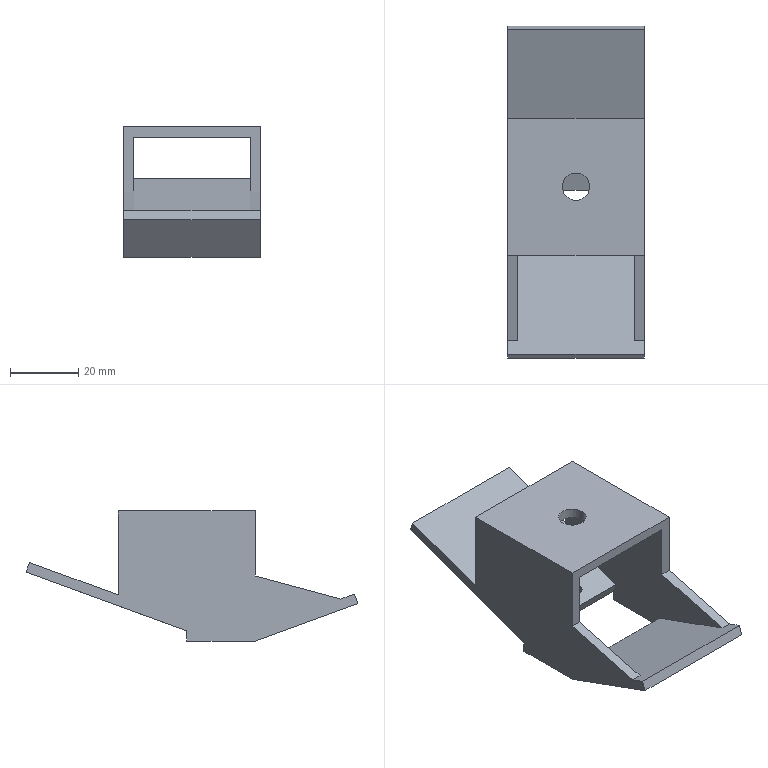Part | STEP file | Blade fixing bracket | 1 solid | 32 faces | box 40 x 96.985 x 38 mm | volume 22805 mm3 | plane 22 | cylinder 10 | commonest cylinder face diameters 2.5 x8 8 x2
STEP:
#1=CARTESIAN_POINT('',(-4.,0.,-1.5));
#2=VERTEX_POINT('',#1);
#3=CARTESIAN_POINT('',(4.,0.,-1.5));
#4=VERTEX_POINT('',#3);
#5=CARTESIAN_POINT('',(0.,0.,-1.5));
#6=DIRECTION('',(0.,0.,1.));
#7=DIRECTION('',(1.,0.,0.));
#8=AXIS2_PLACEMENT_3D('',#5,#6,#7);
#9=CIRCLE('',#8,4.);
#10=EDGE_CURVE('',#2,#4,#9,.T.);
#11=ORIENTED_EDGE('',*,*,#10,.F.);
#12=CARTESIAN_POINT('',(-4.,0.,1.5));
#13=VERTEX_POINT('',#12);
#14=CARTESIAN_POINT('',(-4.,0.,-2.5));
#15=DIRECTION('',(0.,0.,1.));
#16=VECTOR('',#15,1000.);
#17=LINE('',#14,#16);
#18=EDGE_CURVE('',#2,#13,#17,.T.);
#19=ORIENTED_EDGE('',*,*,#18,.T.);
#20=CARTESIAN_POINT('',(4.,0.,1.5));
#21=VERTEX_POINT('',#20);
#22=CARTESIAN_POINT('',(0.,0.,1.5));
#23=DIRECTION('',(0.,0.,1.));
#24=DIRECTION('',(1.,0.,0.));
#25=AXIS2_PLACEMENT_3D('',#22,#23,#24);
#26=CIRCLE('',#25,4.);
#27=EDGE_CURVE('',#13,#21,#26,.T.);
#28=ORIENTED_EDGE('',*,*,#27,.T.);
#29=CARTESIAN_POINT('',(4.,0.,-2.5));
#30=DIRECTION('',(0.,0.,1.));
#31=VECTOR('',#30,1000.);
#32=LINE('',#29,#31);
#33=EDGE_CURVE('',#4,#21,#32,.T.);
#34=ORIENTED_EDGE('',*,*,#33,.F.);
#35=EDGE_LOOP('',(#11,#19,#28,#34));
#36=FACE_OUTER_BOUND('',#35,.T.);
#37=CARTESIAN_POINT('',(0.,0.,-2.5));
#38=DIRECTION('',(0.,0.,1.));
#39=DIRECTION('',(1.,0.,0.));
#40=AXIS2_PLACEMENT_3D('',#37,#38,#39);
#41=CYLINDRICAL_SURFACE('',#40,4.);
#42=ADVANCED_FACE('',(#36),#41,.F.);
#43=CARTESIAN_POINT('',(6.,11.895,-25.978));
#44=VERTEX_POINT('',#43);
#45=CARTESIAN_POINT('',(6.,14.244,-25.123));
#46=VERTEX_POINT('',#45);
#47=CARTESIAN_POINT('',(6.,13.069,-25.551));
#48=DIRECTION('',(0.,0.342,-0.9397));
#49=DIRECTION('',(0.,0.9397,0.342));
#50=AXIS2_PLACEMENT_3D('',#47,#48,#49);
#51=CIRCLE('',#50,1.25);
#52=EDGE_CURVE('',#44,#46,#51,.T.);
#53=ORIENTED_EDGE('',*,*,#52,.F.);
#54=CARTESIAN_POINT('',(6.,12.921,-28.797));
#55=VERTEX_POINT('',#54);
#56=CARTESIAN_POINT('',(6.,12.921,-28.797));
#57=DIRECTION('',(0.,0.342,-0.9397));
#58=VECTOR('',#57,1000.);
#59=LINE('',#56,#58);
#60=EDGE_CURVE('',#44,#55,#59,.T.);
#61=ORIENTED_EDGE('',*,*,#60,.T.);
#62=CARTESIAN_POINT('',(6.,15.27,-27.942));
#63=VERTEX_POINT('',#62);
#64=CARTESIAN_POINT('',(6.,14.095,-28.37));
#65=DIRECTION('',(0.,0.342,-0.9397));
#66=DIRECTION('',(0.,0.9397,0.342));
#67=AXIS2_PLACEMENT_3D('',#64,#65,#66);
#68=CIRCLE('',#67,1.25);
#69=EDGE_CURVE('',#55,#63,#68,.T.);
#70=ORIENTED_EDGE('',*,*,#69,.T.);
#71=CARTESIAN_POINT('',(6.,15.27,-27.942));
#72=DIRECTION('',(0.,0.342,-0.9397));
#73=VECTOR('',#72,1000.);
#74=LINE('',#71,#73);
#75=EDGE_CURVE('',#46,#63,#74,.T.);
#76=ORIENTED_EDGE('',*,*,#75,.F.);
#77=EDGE_LOOP('',(#53,#61,#70,#76));
#78=FACE_OUTER_BOUND('',#77,.T.);
#79=CARTESIAN_POINT('',(6.,14.095,-28.37));
#80=DIRECTION('',(0.,0.342,-0.9397));
#81=DIRECTION('',(0.,0.9397,0.342));
#82=AXIS2_PLACEMENT_3D('',#79,#80,#81);
#83=CYLINDRICAL_SURFACE('',#82,1.25);
#84=ADVANCED_FACE('',(#78),#83,.F.);
#85=CARTESIAN_POINT('',(6.,2.498,-29.398));
#86=VERTEX_POINT('',#85);
#87=CARTESIAN_POINT('',(6.,4.847,-28.543));
#88=VERTEX_POINT('',#87);
#89=CARTESIAN_POINT('',(6.,3.672,-28.971));
#90=DIRECTION('',(0.,0.342,-0.9397));
#91=DIRECTION('',(0.,0.9397,0.342));
#92=AXIS2_PLACEMENT_3D('',#89,#90,#91);
#93=CIRCLE('',#92,1.25);
#94=EDGE_CURVE('',#86,#88,#93,.T.);
#95=ORIENTED_EDGE('',*,*,#94,.F.);
#96=CARTESIAN_POINT('',(6.,3.524,-32.217));
#97=VERTEX_POINT('',#96);
#98=CARTESIAN_POINT('',(6.,3.524,-32.217));
#99=DIRECTION('',(0.,0.342,-0.9397));
#100=VECTOR('',#99,1000.);
#101=LINE('',#98,#100);
#102=EDGE_CURVE('',#86,#97,#101,.T.);
#103=ORIENTED_EDGE('',*,*,#102,.T.);
#104=CARTESIAN_POINT('',(6.,5.873,-31.362));
#105=VERTEX_POINT('',#104);
#106=CARTESIAN_POINT('',(6.,4.698,-31.79));
#107=DIRECTION('',(0.,0.342,-0.9397));
#108=DIRECTION('',(0.,0.9397,0.342));
#109=AXIS2_PLACEMENT_3D('',#106,#107,#108);
#110=CIRCLE('',#109,1.25);
#111=EDGE_CURVE('',#97,#105,#110,.T.);
#112=ORIENTED_EDGE('',*,*,#111,.T.);
#113=CARTESIAN_POINT('',(6.,5.873,-31.362));
#114=DIRECTION('',(0.,0.342,-0.9397));
#115=VECTOR('',#114,1000.);
#116=LINE('',#113,#115);
#117=EDGE_CURVE('',#88,#105,#116,.T.);
#118=ORIENTED_EDGE('',*,*,#117,.F.);
#119=EDGE_LOOP('',(#95,#103,#112,#118));
#120=FACE_OUTER_BOUND('',#119,.T.);
#121=CARTESIAN_POINT('',(6.,4.698,-31.79));
#122=DIRECTION('',(0.,0.342,-0.9397));
#123=DIRECTION('',(0.,0.9397,0.342));
#124=AXIS2_PLACEMENT_3D('',#121,#122,#123);
#125=CYLINDRICAL_SURFACE('',#124,1.25);
#126=ADVANCED_FACE('',(#120),#125,.F.);
#127=CARTESIAN_POINT('',(-6.,2.498,-29.398));
#128=VERTEX_POINT('',#127);
#129=CARTESIAN_POINT('',(-6.,4.847,-28.543));
#130=VERTEX_POINT('',#129);
#131=CARTESIAN_POINT('',(-6.,3.672,-28.971));
#132=DIRECTION('',(0.,0.342,-0.9397));
#133=DIRECTION('',(0.,0.9397,0.342));
#134=AXIS2_PLACEMENT_3D('',#131,#132,#133);
#135=CIRCLE('',#134,1.25);
#136=EDGE_CURVE('',#128,#130,#135,.T.);
#137=ORIENTED_EDGE('',*,*,#136,.F.);
#138=CARTESIAN_POINT('',(-6.,3.524,-32.217));
#139=VERTEX_POINT('',#138);
#140=CARTESIAN_POINT('',(-6.,3.524,-32.217));
#141=DIRECTION('',(0.,0.342,-0.9397));
#142=VECTOR('',#141,1000.);
#143=LINE('',#140,#142);
#144=EDGE_CURVE('',#128,#139,#143,.T.);
#145=ORIENTED_EDGE('',*,*,#144,.T.);
#146=CARTESIAN_POINT('',(-6.,5.873,-31.362));
#147=VERTEX_POINT('',#146);
#148=CARTESIAN_POINT('',(-6.,4.698,-31.79));
#149=DIRECTION('',(0.,0.342,-0.9397));
#150=DIRECTION('',(0.,0.9397,0.342));
#151=AXIS2_PLACEMENT_3D('',#148,#149,#150);
#152=CIRCLE('',#151,1.25);
#153=EDGE_CURVE('',#139,#147,#152,.T.);
#154=ORIENTED_EDGE('',*,*,#153,.T.);
#155=CARTESIAN_POINT('',(-6.,5.873,-31.362));
#156=DIRECTION('',(0.,0.342,-0.9397));
#157=VECTOR('',#156,1000.);
#158=LINE('',#155,#157);
#159=EDGE_CURVE('',#130,#147,#158,.T.);
#160=ORIENTED_EDGE('',*,*,#159,.F.);
#161=EDGE_LOOP('',(#137,#145,#154,#160));
#162=FACE_OUTER_BOUND('',#161,.T.);
#163=CARTESIAN_POINT('',(-6.,4.698,-31.79));
#164=DIRECTION('',(0.,0.342,-0.9397));
#165=DIRECTION('',(0.,0.9397,0.342));
#166=AXIS2_PLACEMENT_3D('',#163,#164,#165);
#167=CYLINDRICAL_SURFACE('',#166,1.25);
#168=ADVANCED_FACE('',(#162),#167,.F.);
#169=CARTESIAN_POINT('',(-6.,11.895,-25.978));
#170=VERTEX_POINT('',#169);
#171=CARTESIAN_POINT('',(-6.,14.244,-25.123));
#172=VERTEX_POINT('',#171);
#173=CARTESIAN_POINT('',(-6.,13.069,-25.551));
#174=DIRECTION('',(0.,0.342,-0.9397));
#175=DIRECTION('',(0.,0.9397,0.342));
#176=AXIS2_PLACEMENT_3D('',#173,#174,#175);
#177=CIRCLE('',#176,1.25);
#178=EDGE_CURVE('',#170,#172,#177,.T.);
#179=ORIENTED_EDGE('',*,*,#178,.F.);
#180=CARTESIAN_POINT('',(-6.,12.921,-28.797));
#181=VERTEX_POINT('',#180);
#182=CARTESIAN_POINT('',(-6.,12.921,-28.797));
#183=DIRECTION('',(0.,0.342,-0.9397));
#184=VECTOR('',#183,1000.);
#185=LINE('',#182,#184);
#186=EDGE_CURVE('',#170,#181,#185,.T.);
#187=ORIENTED_EDGE('',*,*,#186,.T.);
#188=CARTESIAN_POINT('',(-6.,15.27,-27.942));
#189=VERTEX_POINT('',#188);
#190=CARTESIAN_POINT('',(-6.,14.095,-28.37));
#191=DIRECTION('',(0.,0.342,-0.9397));
#192=DIRECTION('',(0.,0.9397,0.342));
#193=AXIS2_PLACEMENT_3D('',#190,#191,#192);
#194=CIRCLE('',#193,1.25);
#195=EDGE_CURVE('',#181,#189,#194,.T.);
#196=ORIENTED_EDGE('',*,*,#195,.T.);
#197=CARTESIAN_POINT('',(-6.,15.27,-27.942));
#198=DIRECTION('',(0.,0.342,-0.9397));
#199=VECTOR('',#198,1000.);
#200=LINE('',#197,#199);
#201=EDGE_CURVE('',#172,#189,#200,.T.);
#202=ORIENTED_EDGE('',*,*,#201,.F.);
#203=EDGE_LOOP('',(#179,#187,#196,#202));
#204=FACE_OUTER_BOUND('',#203,.T.);
#205=CARTESIAN_POINT('',(-6.,14.095,-28.37));
#206=DIRECTION('',(0.,0.342,-0.9397));
#207=DIRECTION('',(0.,0.9397,0.342));
#208=AXIS2_PLACEMENT_3D('',#205,#206,#207);
#209=CYLINDRICAL_SURFACE('',#208,1.25);
#210=ADVANCED_FACE('',(#204),#209,.F.);
#211=CARTESIAN_POINT('',(17.,0.,-33.5));
#212=VERTEX_POINT('',#211);
#213=CARTESIAN_POINT('',(17.,-1.026,-30.681));
#214=VERTEX_POINT('',#213);
#215=CARTESIAN_POINT('',(17.,-1.375,-29.721));
#216=DIRECTION('',(0.,-0.342,0.9397));
#217=VECTOR('',#216,1000.);
#218=LINE('',#215,#217);
#219=EDGE_CURVE('',#212,#214,#218,.T.);
#220=ORIENTED_EDGE('',*,*,#219,.F.);
#221=CARTESIAN_POINT('',(17.,0.,-36.5));
#222=VERTEX_POINT('',#221);
#223=CARTESIAN_POINT('',(17.,0.,-36.5));
#224=DIRECTION('',(0.,0.,-1.));
#225=VECTOR('',#224,1000.);
#226=LINE('',#223,#225);
#227=EDGE_CURVE('',#212,#222,#226,.T.);
#228=ORIENTED_EDGE('',*,*,#227,.T.);
#229=CARTESIAN_POINT('',(17.,-20.,-36.5));
#230=VERTEX_POINT('',#229);
#231=CARTESIAN_POINT('',(17.,-20.,-36.5));
#232=DIRECTION('',(0.,1.,0.));
#233=VECTOR('',#232,1000.);
#234=LINE('',#231,#233);
#235=EDGE_CURVE('',#230,#222,#234,.T.);
#236=ORIENTED_EDGE('',*,*,#235,.F.);
#237=CARTESIAN_POINT('',(17.,-18.974,-33.681));
#238=VERTEX_POINT('',#237);
#239=CARTESIAN_POINT('',(17.,-20.,-36.5));
#240=DIRECTION('',(0.,-0.342,-0.9397));
#241=VECTOR('',#240,1000.);
#242=LINE('',#239,#241);
#243=EDGE_CURVE('',#238,#230,#242,.T.);
#244=ORIENTED_EDGE('',*,*,#243,.F.);
#245=CARTESIAN_POINT('',(17.,-44.959,-24.223));
#246=VERTEX_POINT('',#245);
#247=CARTESIAN_POINT('',(17.,-18.974,-33.681));
#248=DIRECTION('',(0.,0.9397,-0.342));
#249=VECTOR('',#248,1000.);
#250=LINE('',#247,#249);
#251=EDGE_CURVE('',#246,#238,#250,.T.);
#252=ORIENTED_EDGE('',*,*,#251,.F.);
#253=CARTESIAN_POINT('',(17.,-20.,-17.5));
#254=VERTEX_POINT('',#253);
#255=CARTESIAN_POINT('',(17.,-50.,-25.581));
#256=DIRECTION('',(0.,-0.9656,-0.2601));
#257=VECTOR('',#256,1000.);
#258=LINE('',#255,#257);
#259=EDGE_CURVE('',#254,#246,#258,.T.);
#260=ORIENTED_EDGE('',*,*,#259,.F.);
#261=CARTESIAN_POINT('',(17.,-20.,-1.5));
#262=VERTEX_POINT('',#261);
#263=CARTESIAN_POINT('',(17.,-20.,-36.5));
#264=DIRECTION('',(0.,0.,1.));
#265=VECTOR('',#264,1000.);
#266=LINE('',#263,#265);
#267=EDGE_CURVE('',#254,#262,#266,.T.);
#268=ORIENTED_EDGE('',*,*,#267,.T.);
#269=CARTESIAN_POINT('',(17.,20.,-1.5));
#270=VERTEX_POINT('',#269);
#271=CARTESIAN_POINT('',(17.,-20.,-1.5));
#272=DIRECTION('',(0.,1.,0.));
#273=VECTOR('',#272,1000.);
#274=LINE('',#271,#273);
#275=EDGE_CURVE('',#262,#270,#274,.T.);
#276=ORIENTED_EDGE('',*,*,#275,.T.);
#277=CARTESIAN_POINT('',(17.,20.,-23.028));
#278=VERTEX_POINT('',#277);
#279=CARTESIAN_POINT('',(17.,20.,-36.5));
#280=DIRECTION('',(0.,0.,1.));
#281=VECTOR('',#280,1000.);
#282=LINE('',#279,#281);
#283=EDGE_CURVE('',#278,#270,#282,.T.);
#284=ORIENTED_EDGE('',*,*,#283,.F.);
#285=CARTESIAN_POINT('',(17.,-19.651,-37.46));
#286=DIRECTION('',(0.,0.9397,0.342));
#287=VECTOR('',#286,1000.);
#288=LINE('',#285,#287);
#289=EDGE_CURVE('',#214,#278,#288,.T.);
#290=ORIENTED_EDGE('',*,*,#289,.F.);
#291=EDGE_LOOP('',(#220,#228,#236,#244,#252,#260,#268,#276,#284,#290));
#292=FACE_OUTER_BOUND('',#291,.T.);
#293=CARTESIAN_POINT('',(17.,-20.,-36.5));
#294=DIRECTION('',(1.,0.,0.));
#295=DIRECTION('',(0.,0.,-1.));
#296=AXIS2_PLACEMENT_3D('',#293,#294,#295);
#297=PLANE('',#296);
#298=ADVANCED_FACE('',(#292),#297,.F.);
#299=CARTESIAN_POINT('',(-17.,0.,-36.5));
#300=VERTEX_POINT('',#299);
#301=CARTESIAN_POINT('',(-17.,-20.,-36.5));
#302=VERTEX_POINT('',#301);
#303=CARTESIAN_POINT('',(-17.,-20.,-36.5));
#304=DIRECTION('',(0.,-1.,0.));
#305=VECTOR('',#304,1000.);
#306=LINE('',#303,#305);
#307=EDGE_CURVE('',#300,#302,#306,.T.);
#308=ORIENTED_EDGE('',*,*,#307,.F.);
#309=CARTESIAN_POINT('',(-17.,0.,-33.5));
#310=VERTEX_POINT('',#309);
#311=CARTESIAN_POINT('',(-17.,0.,-36.5));
#312=DIRECTION('',(0.,0.,1.));
#313=VECTOR('',#312,1000.);
#314=LINE('',#311,#313);
#315=EDGE_CURVE('',#300,#310,#314,.T.);
#316=ORIENTED_EDGE('',*,*,#315,.T.);
#317=CARTESIAN_POINT('',(-17.,-1.026,-30.681));
#318=VERTEX_POINT('',#317);
#319=CARTESIAN_POINT('',(-17.,-1.375,-29.721));
#320=DIRECTION('',(0.,0.342,-0.9397));
#321=VECTOR('',#320,1000.);
#322=LINE('',#319,#321);
#323=EDGE_CURVE('',#318,#310,#322,.T.);
#324=ORIENTED_EDGE('',*,*,#323,.F.);
#325=CARTESIAN_POINT('',(-17.,20.,-23.028));
#326=VERTEX_POINT('',#325);
#327=CARTESIAN_POINT('',(-17.,-19.651,-37.46));
#328=DIRECTION('',(0.,-0.9397,-0.342));
#329=VECTOR('',#328,1000.);
#330=LINE('',#327,#329);
#331=EDGE_CURVE('',#326,#318,#330,.T.);
#332=ORIENTED_EDGE('',*,*,#331,.F.);
#333=CARTESIAN_POINT('',(-17.,20.,-1.5));
#334=VERTEX_POINT('',#333);
#335=CARTESIAN_POINT('',(-17.,20.,-36.5));
#336=DIRECTION('',(0.,0.,1.));
#337=VECTOR('',#336,1000.);
#338=LINE('',#335,#337);
#339=EDGE_CURVE('',#326,#334,#338,.T.);
#340=ORIENTED_EDGE('',*,*,#339,.T.);
#341=CARTESIAN_POINT('',(-17.,-20.,-1.5));
#342=VERTEX_POINT('',#341);
#343=CARTESIAN_POINT('',(-17.,-20.,-1.5));
#344=DIRECTION('',(0.,-1.,0.));
#345=VECTOR('',#344,1000.);
#346=LINE('',#343,#345);
#347=EDGE_CURVE('',#334,#342,#346,.T.);
#348=ORIENTED_EDGE('',*,*,#347,.T.);
#349=CARTESIAN_POINT('',(-17.,-20.,-17.5));
#350=VERTEX_POINT('',#349);
#351=CARTESIAN_POINT('',(-17.,-20.,-36.5));
#352=DIRECTION('',(0.,0.,1.));
#353=VECTOR('',#352,1000.);
#354=LINE('',#351,#353);
#355=EDGE_CURVE('',#350,#342,#354,.T.);
#356=ORIENTED_EDGE('',*,*,#355,.F.);
#357=CARTESIAN_POINT('',(-17.,-44.959,-24.223));
#358=VERTEX_POINT('',#357);
#359=CARTESIAN_POINT('',(-17.,-50.,-25.581));
#360=DIRECTION('',(0.,-0.9656,-0.2601));
#361=VECTOR('',#360,1000.);
#362=LINE('',#359,#361);
#363=EDGE_CURVE('',#350,#358,#362,.T.);
#364=ORIENTED_EDGE('',*,*,#363,.T.);
#365=CARTESIAN_POINT('',(-17.,-18.974,-33.681));
#366=VERTEX_POINT('',#365);
#367=CARTESIAN_POINT('',(-17.,-18.974,-33.681));
#368=DIRECTION('',(0.,-0.9397,0.342));
#369=VECTOR('',#368,1000.);
#370=LINE('',#367,#369);
#371=EDGE_CURVE('',#366,#358,#370,.T.);
#372=ORIENTED_EDGE('',*,*,#371,.F.);
#373=CARTESIAN_POINT('',(-17.,-20.,-36.5));
#374=DIRECTION('',(0.,0.342,0.9397));
#375=VECTOR('',#374,1000.);
#376=LINE('',#373,#375);
#377=EDGE_CURVE('',#302,#366,#376,.T.);
#378=ORIENTED_EDGE('',*,*,#377,.F.);
#379=EDGE_LOOP('',(#308,#316,#324,#332,#340,#348,#356,#364,#372,#378));
#380=FACE_OUTER_BOUND('',#379,.T.);
#381=CARTESIAN_POINT('',(-17.,-20.,-36.5));
#382=DIRECTION('',(-1.,0.,0.));
#383=DIRECTION('',(0.,0.,1.));
#384=AXIS2_PLACEMENT_3D('',#381,#382,#383);
#385=PLANE('',#384);
#386=ADVANCED_FACE('',(#380),#385,.F.);
#387=CARTESIAN_POINT('',(-20.,20.,-23.028));
#388=VERTEX_POINT('',#387);
#389=CARTESIAN_POINT('',(-20.,20.,-23.028));
#390=DIRECTION('',(1.,0.,0.));
#391=VECTOR('',#390,1000.);
#392=LINE('',#389,#391);
#393=EDGE_CURVE('',#388,#326,#392,.T.);
#394=ORIENTED_EDGE('',*,*,#393,.F.);
#395=CARTESIAN_POINT('',(-20.,20.,1.5));
#396=VERTEX_POINT('',#395);
#397=CARTESIAN_POINT('',(-20.,20.,1.5));
#398=DIRECTION('',(0.,0.,-1.));
#399=VECTOR('',#398,1000.);
#400=LINE('',#397,#399);
#401=EDGE_CURVE('',#396,#388,#400,.T.);
#402=ORIENTED_EDGE('',*,*,#401,.F.);
#403=CARTESIAN_POINT('',(20.,20.,1.5));
#404=VERTEX_POINT('',#403);
#405=CARTESIAN_POINT('',(-20.,20.,1.5));
#406=DIRECTION('',(-1.,0.,0.));
#407=VECTOR('',#406,1000.);
#408=LINE('',#405,#407);
#409=EDGE_CURVE('',#404,#396,#408,.T.);
#410=ORIENTED_EDGE('',*,*,#409,.F.);
#411=CARTESIAN_POINT('',(20.,20.,-23.028));
#412=VERTEX_POINT('',#411);
#413=CARTESIAN_POINT('',(20.,20.,1.5));
#414=DIRECTION('',(0.,0.,-1.));
#415=VECTOR('',#414,1000.);
#416=LINE('',#413,#415);
#417=EDGE_CURVE('',#404,#412,#416,.T.);
#418=ORIENTED_EDGE('',*,*,#417,.T.);
#419=CARTESIAN_POINT('',(-20.,20.,-23.028));
#420=DIRECTION('',(1.,0.,0.));
#421=VECTOR('',#420,1000.);
#422=LINE('',#419,#421);
#423=EDGE_CURVE('',#278,#412,#422,.T.);
#424=ORIENTED_EDGE('',*,*,#423,.F.);
#425=ORIENTED_EDGE('',*,*,#283,.T.);
#426=CARTESIAN_POINT('',(-20.,20.,-1.5));
#427=DIRECTION('',(-1.,0.,0.));
#428=VECTOR('',#427,1000.);
#429=LINE('',#426,#428);
#430=EDGE_CURVE('',#270,#334,#429,.T.);
#431=ORIENTED_EDGE('',*,*,#430,.T.);
#432=ORIENTED_EDGE('',*,*,#339,.F.);
#433=EDGE_LOOP('',(#394,#402,#410,#418,#424,#425,#431,#432));
#434=FACE_OUTER_BOUND('',#433,.T.);
#435=CARTESIAN_POINT('',(-20.,20.,1.5));
#436=DIRECTION('',(0.,-1.,0.));
#437=DIRECTION('',(0.,0.,-1.));
#438=AXIS2_PLACEMENT_3D('',#435,#436,#437);
#439=PLANE('',#438);
#440=ADVANCED_FACE('',(#434),#439,.F.);
#441=ORIENTED_EDGE('',*,*,#259,.T.);
#442=CARTESIAN_POINT('',(20.,-44.959,-24.223));
#443=VERTEX_POINT('',#442);
#444=CARTESIAN_POINT('',(17.,-44.959,-24.223));
#445=DIRECTION('',(1.,0.,0.));
#446=VECTOR('',#445,1000.);
#447=LINE('',#444,#446);
#448=EDGE_CURVE('',#246,#443,#447,.T.);
#449=ORIENTED_EDGE('',*,*,#448,.T.);
#450=CARTESIAN_POINT('',(20.,-20.,-17.5));
#451=VERTEX_POINT('',#450);
#452=CARTESIAN_POINT('',(20.,-50.,-25.581));
#453=DIRECTION('',(0.,-0.9656,-0.2601));
#454=VECTOR('',#453,1000.);
#455=LINE('',#452,#454);
#456=EDGE_CURVE('',#451,#443,#455,.T.);
#457=ORIENTED_EDGE('',*,*,#456,.F.);
#458=CARTESIAN_POINT('',(17.,-20.,-17.5));
#459=DIRECTION('',(1.,0.,0.));
#460=VECTOR('',#459,1000.);
#461=LINE('',#458,#460);
#462=EDGE_CURVE('',#254,#451,#461,.T.);
#463=ORIENTED_EDGE('',*,*,#462,.F.);
#464=EDGE_LOOP('',(#441,#449,#457,#463));
#465=FACE_OUTER_BOUND('',#464,.T.);
#466=CARTESIAN_POINT('',(17.,-50.,-25.581));
#467=DIRECTION('',(0.,-0.2601,0.9656));
#468=DIRECTION('',(0.,-0.9656,-0.2601));
#469=AXIS2_PLACEMENT_3D('',#466,#467,#468);
#470=PLANE('',#469);
#471=ADVANCED_FACE('',(#465),#470,.T.);
#472=CARTESIAN_POINT('',(-20.,-44.959,-24.223));
#473=VERTEX_POINT('',#472);
#474=CARTESIAN_POINT('',(-17.,-44.959,-24.223));
#475=DIRECTION('',(-1.,0.,0.));
#476=VECTOR('',#475,1000.);
#477=LINE('',#474,#476);
#478=EDGE_CURVE('',#358,#473,#477,.T.);
#479=ORIENTED_EDGE('',*,*,#478,.F.);
#480=ORIENTED_EDGE('',*,*,#363,.F.);
#481=CARTESIAN_POINT('',(-20.,-20.,-17.5));
#482=VERTEX_POINT('',#481);
#483=CARTESIAN_POINT('',(-17.,-20.,-17.5));
#484=DIRECTION('',(-1.,0.,0.));
#485=VECTOR('',#484,1000.);
#486=LINE('',#483,#485);
#487=EDGE_CURVE('',#350,#482,#486,.T.);
#488=ORIENTED_EDGE('',*,*,#487,.T.);
#489=CARTESIAN_POINT('',(-20.,-50.,-25.581));
#490=DIRECTION('',(0.,-0.9656,-0.2601));
#491=VECTOR('',#490,1000.);
#492=LINE('',#489,#491);
#493=EDGE_CURVE('',#482,#473,#492,.T.);
#494=ORIENTED_EDGE('',*,*,#493,.T.);
#495=EDGE_LOOP('',(#479,#480,#488,#494));
#496=FACE_OUTER_BOUND('',#495,.T.);
#497=CARTESIAN_POINT('',(-17.,-50.,-25.581));
#498=DIRECTION('',(0.,0.2601,-0.9656));
#499=DIRECTION('',(0.,0.9656,0.2601));
#500=AXIS2_PLACEMENT_3D('',#497,#498,#499);
#501=PLANE('',#500);
#502=ADVANCED_FACE('',(#496),#501,.F.);
#503=ORIENTED_EDGE('',*,*,#487,.F.);
#504=ORIENTED_EDGE('',*,*,#355,.T.);
#505=CARTESIAN_POINT('',(-20.,-20.,-1.5));
#506=DIRECTION('',(1.,0.,0.));
#507=VECTOR('',#506,1000.);
#508=LINE('',#505,#507);
#509=EDGE_CURVE('',#342,#262,#508,.T.);
#510=ORIENTED_EDGE('',*,*,#509,.T.);
#511=ORIENTED_EDGE('',*,*,#267,.F.);
#512=ORIENTED_EDGE('',*,*,#462,.T.);
#513=CARTESIAN_POINT('',(20.,-20.,1.5));
#514=VERTEX_POINT('',#513);
#515=CARTESIAN_POINT('',(20.,-20.,1.5));
#516=DIRECTION('',(0.,0.,-1.));
#517=VECTOR('',#516,1000.);
#518=LINE('',#515,#517);
#519=EDGE_CURVE('',#514,#451,#518,.T.);
#520=ORIENTED_EDGE('',*,*,#519,.F.);
#521=CARTESIAN_POINT('',(-20.,-20.,1.5));
#522=VERTEX_POINT('',#521);
#523=CARTESIAN_POINT('',(-20.,-20.,1.5));
#524=DIRECTION('',(1.,0.,0.));
#525=VECTOR('',#524,1000.);
#526=LINE('',#523,#525);
#527=EDGE_CURVE('',#522,#514,#526,.T.);
#528=ORIENTED_EDGE('',*,*,#527,.F.);
#529=CARTESIAN_POINT('',(-20.,-20.,1.5));
#530=DIRECTION('',(0.,0.,-1.));
#531=VECTOR('',#530,1000.);
#532=LINE('',#529,#531);
#533=EDGE_CURVE('',#522,#482,#532,.T.);
#534=ORIENTED_EDGE('',*,*,#533,.T.);
#535=EDGE_LOOP('',(#503,#504,#510,#511,#512,#520,#528,#534));
#536=FACE_OUTER_BOUND('',#535,.T.);
#537=CARTESIAN_POINT('',(-20.,-20.,1.5));
#538=DIRECTION('',(0.,1.,0.));
#539=DIRECTION('',(0.,0.,1.));
#540=AXIS2_PLACEMENT_3D('',#537,#538,#539);
#541=PLANE('',#540);
#542=ADVANCED_FACE('',(#536),#541,.F.);
#543=CARTESIAN_POINT('',(0.,0.,-1.5));
#544=DIRECTION('',(0.,0.,1.));
#545=DIRECTION('',(1.,0.,0.));
#546=AXIS2_PLACEMENT_3D('',#543,#544,#545);
#547=CIRCLE('',#546,4.);
#548=EDGE_CURVE('',#4,#2,#547,.T.);
#549=ORIENTED_EDGE('',*,*,#548,.T.);
#550=ORIENTED_EDGE('',*,*,#10,.T.);
#551=EDGE_LOOP('',(#549,#550));
#552=FACE_BOUND('',#551,.T.);
#553=ORIENTED_EDGE('',*,*,#347,.F.);
#554=ORIENTED_EDGE('',*,*,#430,.F.);
#555=ORIENTED_EDGE('',*,*,#275,.F.);
#556=ORIENTED_EDGE('',*,*,#509,.F.);
#557=EDGE_LOOP('',(#553,#554,#555,#556));
#558=FACE_OUTER_BOUND('',#557,.T.);
#559=CARTESIAN_POINT('',(0.,0.,-1.5));
#560=DIRECTION('',(0.,0.,1.));
#561=DIRECTION('',(1.,0.,0.));
#562=AXIS2_PLACEMENT_3D('',#559,#560,#561);
#563=PLANE('',#562);
#564=ADVANCED_FACE('',(#552,#558),#563,.F.);
#565=CARTESIAN_POINT('',(20.,0.,-36.5));
#566=VERTEX_POINT('',#565);
#567=CARTESIAN_POINT('',(20.,0.,-33.5));
#568=VERTEX_POINT('',#567);
#569=CARTESIAN_POINT('',(20.,0.,1.5));
#570=DIRECTION('',(0.,0.,1.));
#571=VECTOR('',#570,1000.);
#572=LINE('',#569,#571);
#573=EDGE_CURVE('',#566,#568,#572,.T.);
#574=ORIENTED_EDGE('',*,*,#573,.T.);
#575=CARTESIAN_POINT('',(20.,46.985,-16.399));
#576=VERTEX_POINT('',#575);
#577=CARTESIAN_POINT('',(20.,46.985,-16.399));
#578=DIRECTION('',(0.,-0.9397,-0.342));
#579=VECTOR('',#578,1000.);
#580=LINE('',#577,#579);
#581=EDGE_CURVE('',#576,#568,#580,.T.);
#582=ORIENTED_EDGE('',*,*,#581,.F.);
#583=CARTESIAN_POINT('',(20.,45.959,-13.58));
#584=VERTEX_POINT('',#583);
#585=CARTESIAN_POINT('',(20.,45.959,-13.58));
#586=DIRECTION('',(0.,0.342,-0.9397));
#587=VECTOR('',#586,1000.);
#588=LINE('',#585,#587);
#589=EDGE_CURVE('',#584,#576,#588,.T.);
#590=ORIENTED_EDGE('',*,*,#589,.F.);
#591=CARTESIAN_POINT('',(20.,-1.026,-30.681));
#592=DIRECTION('',(0.,0.9397,0.342));
#593=VECTOR('',#592,1000.);
#594=LINE('',#591,#593);
#595=EDGE_CURVE('',#412,#584,#594,.T.);
#596=ORIENTED_EDGE('',*,*,#595,.F.);
#597=ORIENTED_EDGE('',*,*,#417,.F.);
#598=CARTESIAN_POINT('',(20.,20.,1.5));
#599=DIRECTION('',(0.,1.,0.));
#600=VECTOR('',#599,1000.);
#601=LINE('',#598,#600);
#602=EDGE_CURVE('',#514,#404,#601,.T.);
#603=ORIENTED_EDGE('',*,*,#602,.F.);
#604=ORIENTED_EDGE('',*,*,#519,.T.);
#605=ORIENTED_EDGE('',*,*,#456,.T.);
#606=CARTESIAN_POINT('',(20.,-48.974,-22.762));
#607=VERTEX_POINT('',#606);
#608=CARTESIAN_POINT('',(20.,-48.974,-22.762));
#609=DIRECTION('',(0.,-0.9397,0.342));
#610=VECTOR('',#609,1000.);
#611=LINE('',#608,#610);
#612=EDGE_CURVE('',#443,#607,#611,.T.);
#613=ORIENTED_EDGE('',*,*,#612,.T.);
#614=CARTESIAN_POINT('',(20.,-50.,-25.581));
#615=VERTEX_POINT('',#614);
#616=CARTESIAN_POINT('',(20.,-48.974,-22.762));
#617=DIRECTION('',(0.,-0.342,-0.9397));
#618=VECTOR('',#617,1000.);
#619=LINE('',#616,#618);
#620=EDGE_CURVE('',#607,#615,#619,.T.);
#621=ORIENTED_EDGE('',*,*,#620,.T.);
#622=CARTESIAN_POINT('',(20.,-20.,-36.5));
#623=VERTEX_POINT('',#622);
#624=CARTESIAN_POINT('',(20.,-20.,-36.5));
#625=DIRECTION('',(0.,0.9397,-0.342));
#626=VECTOR('',#625,1000.);
#627=LINE('',#624,#626);
#628=EDGE_CURVE('',#615,#623,#627,.T.);
#629=ORIENTED_EDGE('',*,*,#628,.T.);
#630=CARTESIAN_POINT('',(20.,-20.,-36.5));
#631=DIRECTION('',(0.,-1.,0.));
#632=VECTOR('',#631,1000.);
#633=LINE('',#630,#632);
#634=EDGE_CURVE('',#566,#623,#633,.T.);
#635=ORIENTED_EDGE('',*,*,#634,.F.);
#636=EDGE_LOOP('',(#574,#582,#590,#596,#597,#603,#604,#605,#613,#621,#629,#635));
#637=FACE_OUTER_BOUND('',#636,.T.);
#638=CARTESIAN_POINT('',(20.,20.,1.5));
#639=DIRECTION('',(-1.,0.,0.));
#640=DIRECTION('',(0.,-1.,0.));
#641=AXIS2_PLACEMENT_3D('',#638,#639,#640);
#642=PLANE('',#641);
#643=ADVANCED_FACE('',(#637),#642,.F.);
#644=CARTESIAN_POINT('',(-20.,0.,-33.5));
#645=VERTEX_POINT('',#644);
#646=CARTESIAN_POINT('',(-20.,46.985,-16.399));
#647=VERTEX_POINT('',#646);
#648=CARTESIAN_POINT('',(-20.,0.,-33.5));
#649=DIRECTION('',(0.,0.9397,0.342));
#650=VECTOR('',#649,1000.);
#651=LINE('',#648,#650);
#652=EDGE_CURVE('',#645,#647,#651,.T.);
#653=ORIENTED_EDGE('',*,*,#652,.F.);
#654=CARTESIAN_POINT('',(-20.,0.,-36.5));
#655=VERTEX_POINT('',#654);
#656=CARTESIAN_POINT('',(-20.,0.,1.5));
#657=DIRECTION('',(0.,0.,-1.));
#658=VECTOR('',#657,1000.);
#659=LINE('',#656,#658);
#660=EDGE_CURVE('',#645,#655,#659,.T.);
#661=ORIENTED_EDGE('',*,*,#660,.T.);
#662=CARTESIAN_POINT('',(-20.,-20.,-36.5));
#663=VERTEX_POINT('',#662);
#664=CARTESIAN_POINT('',(-20.,-20.,-36.5));
#665=DIRECTION('',(0.,1.,0.));
#666=VECTOR('',#665,1000.);
#667=LINE('',#664,#666);
#668=EDGE_CURVE('',#663,#655,#667,.T.);
#669=ORIENTED_EDGE('',*,*,#668,.F.);
#670=CARTESIAN_POINT('',(-20.,-50.,-25.581));
#671=VERTEX_POINT('',#670);
#672=CARTESIAN_POINT('',(-20.,-20.,-36.5));
#673=DIRECTION('',(0.,0.9397,-0.342));
#674=VECTOR('',#673,1000.);
#675=LINE('',#672,#674);
#676=EDGE_CURVE('',#671,#663,#675,.T.);
#677=ORIENTED_EDGE('',*,*,#676,.F.);
#678=CARTESIAN_POINT('',(-20.,-48.974,-22.762));
#679=VERTEX_POINT('',#678);
#680=CARTESIAN_POINT('',(-20.,-48.974,-22.762));
#681=DIRECTION('',(0.,-0.342,-0.9397));
#682=VECTOR('',#681,1000.);
#683=LINE('',#680,#682);
#684=EDGE_CURVE('',#679,#671,#683,.T.);
#685=ORIENTED_EDGE('',*,*,#684,.F.);
#686=CARTESIAN_POINT('',(-20.,-48.974,-22.762));
#687=DIRECTION('',(0.,-0.9397,0.342));
#688=VECTOR('',#687,1000.);
#689=LINE('',#686,#688);
#690=EDGE_CURVE('',#473,#679,#689,.T.);
#691=ORIENTED_EDGE('',*,*,#690,.F.);
#692=ORIENTED_EDGE('',*,*,#493,.F.);
#693=ORIENTED_EDGE('',*,*,#533,.F.);
#694=CARTESIAN_POINT('',(-20.,20.,1.5));
#695=DIRECTION('',(0.,-1.,0.));
#696=VECTOR('',#695,1000.);
#697=LINE('',#694,#696);
#698=EDGE_CURVE('',#396,#522,#697,.T.);
#699=ORIENTED_EDGE('',*,*,#698,.F.);
#700=ORIENTED_EDGE('',*,*,#401,.T.);
#701=CARTESIAN_POINT('',(-20.,45.959,-13.58));
#702=VERTEX_POINT('',#701);
#703=CARTESIAN_POINT('',(-20.,-1.026,-30.681));
#704=DIRECTION('',(0.,-0.9397,-0.342));
#705=VECTOR('',#704,1000.);
#706=LINE('',#703,#705);
#707=EDGE_CURVE('',#702,#388,#706,.T.);
#708=ORIENTED_EDGE('',*,*,#707,.F.);
#709=CARTESIAN_POINT('',(-20.,45.959,-13.58));
#710=DIRECTION('',(0.,-0.342,0.9397));
#711=VECTOR('',#710,1000.);
#712=LINE('',#709,#711);
#713=EDGE_CURVE('',#647,#702,#712,.T.);
#714=ORIENTED_EDGE('',*,*,#713,.F.);
#715=EDGE_LOOP('',(#653,#661,#669,#677,#685,#691,#692,#693,#699,#700,#708,#714));
#716=FACE_OUTER_BOUND('',#715,.T.);
#717=CARTESIAN_POINT('',(-20.,20.,1.5));
#718=DIRECTION('',(1.,0.,0.));
#719=DIRECTION('',(0.,1.,0.));
#720=AXIS2_PLACEMENT_3D('',#717,#718,#719);
#721=PLANE('',#720);
#722=ADVANCED_FACE('',(#716),#721,.F.);
#723=CARTESIAN_POINT('',(0.,0.,1.5));
#724=DIRECTION('',(0.,0.,1.));
#725=DIRECTION('',(1.,0.,0.));
#726=AXIS2_PLACEMENT_3D('',#723,#724,#725);
#727=CIRCLE('',#726,4.);
#728=EDGE_CURVE('',#21,#13,#727,.T.);
#729=ORIENTED_EDGE('',*,*,#728,.F.);
#730=ORIENTED_EDGE('',*,*,#27,.F.);
#731=EDGE_LOOP('',(#729,#730));
#732=FACE_BOUND('',#731,.T.);
#733=ORIENTED_EDGE('',*,*,#602,.T.);
#734=ORIENTED_EDGE('',*,*,#409,.T.);
#735=ORIENTED_EDGE('',*,*,#698,.T.);
#736=ORIENTED_EDGE('',*,*,#527,.T.);
#737=EDGE_LOOP('',(#733,#734,#735,#736));
#738=FACE_OUTER_BOUND('',#737,.T.);
#739=CARTESIAN_POINT('',(0.,0.,1.5));
#740=DIRECTION('',(0.,0.,1.));
#741=DIRECTION('',(1.,0.,0.));
#742=AXIS2_PLACEMENT_3D('',#739,#740,#741);
#743=PLANE('',#742);
#744=ADVANCED_FACE('',(#732,#738),#743,.T.);
#745=ORIENTED_EDGE('',*,*,#235,.T.);
#746=CARTESIAN_POINT('',(0.,0.,-36.5));
#747=DIRECTION('',(1.,0.,0.));
#748=VECTOR('',#747,1000.);
#749=LINE('',#746,#748);
#750=EDGE_CURVE('',#222,#566,#749,.T.);
#751=ORIENTED_EDGE('',*,*,#750,.T.);
#752=ORIENTED_EDGE('',*,*,#634,.T.);
#753=CARTESIAN_POINT('',(20.,-20.,-36.5));
#754=DIRECTION('',(-1.,0.,0.));
#755=VECTOR('',#754,1000.);
#756=LINE('',#753,#755);
#757=EDGE_CURVE('',#623,#230,#756,.T.);
#758=ORIENTED_EDGE('',*,*,#757,.T.);
#759=EDGE_LOOP('',(#745,#751,#752,#758));
#760=FACE_OUTER_BOUND('',#759,.T.);
#761=CARTESIAN_POINT('',(0.,0.,-36.5));
#762=DIRECTION('',(0.,0.,1.));
#763=DIRECTION('',(1.,0.,0.));
#764=AXIS2_PLACEMENT_3D('',#761,#762,#763);
#765=PLANE('',#764);
#766=ADVANCED_FACE('',(#760),#765,.F.);
#767=CARTESIAN_POINT('',(0.,0.,-36.5));
#768=DIRECTION('',(-1.,0.,0.));
#769=VECTOR('',#768,1000.);
#770=LINE('',#767,#769);
#771=EDGE_CURVE('',#300,#655,#770,.T.);
#772=ORIENTED_EDGE('',*,*,#771,.F.);
#773=ORIENTED_EDGE('',*,*,#307,.T.);
#774=CARTESIAN_POINT('',(-20.,-20.,-36.5));
#775=DIRECTION('',(-1.,0.,0.));
#776=VECTOR('',#775,1000.);
#777=LINE('',#774,#776);
#778=EDGE_CURVE('',#302,#663,#777,.T.);
#779=ORIENTED_EDGE('',*,*,#778,.T.);
#780=ORIENTED_EDGE('',*,*,#668,.T.);
#781=EDGE_LOOP('',(#772,#773,#779,#780));
#782=FACE_OUTER_BOUND('',#781,.T.);
#783=CARTESIAN_POINT('',(0.,0.,-36.5));
#784=DIRECTION('',(0.,0.,-1.));
#785=DIRECTION('',(-1.,0.,0.));
#786=AXIS2_PLACEMENT_3D('',#783,#784,#785);
#787=PLANE('',#786);
#788=ADVANCED_FACE('',(#782),#787,.T.);
#789=ORIENTED_EDGE('',*,*,#628,.F.);
#790=CARTESIAN_POINT('',(17.,-50.,-25.581));
#791=DIRECTION('',(1.,0.,0.));
#792=VECTOR('',#791,1000.);
#793=LINE('',#790,#792);
#794=EDGE_CURVE('',#671,#615,#793,.T.);
#795=ORIENTED_EDGE('',*,*,#794,.F.);
#796=ORIENTED_EDGE('',*,*,#676,.T.);
#797=ORIENTED_EDGE('',*,*,#778,.F.);
#798=CARTESIAN_POINT('',(20.,-20.,-36.5));
#799=DIRECTION('',(-1.,0.,0.));
#800=VECTOR('',#799,1000.);
#801=LINE('',#798,#800);
#802=EDGE_CURVE('',#230,#302,#801,.T.);
#803=ORIENTED_EDGE('',*,*,#802,.F.);
#804=ORIENTED_EDGE('',*,*,#757,.F.);
#805=EDGE_LOOP('',(#789,#795,#796,#797,#803,#804));
#806=FACE_OUTER_BOUND('',#805,.T.);
#807=CARTESIAN_POINT('',(17.,-20.,-36.5));
#808=DIRECTION('',(0.,-0.342,-0.9397));
#809=DIRECTION('',(0.,0.9397,-0.342));
#810=AXIS2_PLACEMENT_3D('',#807,#808,#809);
#811=PLANE('',#810);
#812=ADVANCED_FACE('',(#806),#811,.T.);
#813=ORIENTED_EDGE('',*,*,#448,.F.);
#814=ORIENTED_EDGE('',*,*,#251,.T.);
#815=CARTESIAN_POINT('',(20.,-18.974,-33.681));
#816=DIRECTION('',(-1.,0.,0.));
#817=VECTOR('',#816,1000.);
#818=LINE('',#815,#817);
#819=EDGE_CURVE('',#238,#366,#818,.T.);
#820=ORIENTED_EDGE('',*,*,#819,.T.);
#821=ORIENTED_EDGE('',*,*,#371,.T.);
#822=ORIENTED_EDGE('',*,*,#478,.T.);
#823=ORIENTED_EDGE('',*,*,#690,.T.);
#824=CARTESIAN_POINT('',(20.,-48.974,-22.762));
#825=DIRECTION('',(-1.,0.,0.));
#826=VECTOR('',#825,1000.);
#827=LINE('',#824,#826);
#828=EDGE_CURVE('',#607,#679,#827,.T.);
#829=ORIENTED_EDGE('',*,*,#828,.F.);
#830=ORIENTED_EDGE('',*,*,#612,.F.);
#831=EDGE_LOOP('',(#813,#814,#820,#821,#822,#823,#829,#830));
#832=FACE_OUTER_BOUND('',#831,.T.);
#833=CARTESIAN_POINT('',(20.,-48.974,-22.762));
#834=DIRECTION('',(0.,-0.342,-0.9397));
#835=DIRECTION('',(0.,0.9397,-0.342));
#836=AXIS2_PLACEMENT_3D('',#833,#834,#835);
#837=PLANE('',#836);
#838=ADVANCED_FACE('',(#832),#837,.F.);
#839=ORIENTED_EDGE('',*,*,#819,.F.);
#840=ORIENTED_EDGE('',*,*,#243,.T.);
#841=ORIENTED_EDGE('',*,*,#802,.T.);
#842=ORIENTED_EDGE('',*,*,#377,.T.);
#843=EDGE_LOOP('',(#839,#840,#841,#842));
#844=FACE_OUTER_BOUND('',#843,.T.);
#845=CARTESIAN_POINT('',(20.,-18.974,-33.681));
#846=DIRECTION('',(0.,-0.9397,0.342));
#847=DIRECTION('',(0.,-0.342,-0.9397));
#848=AXIS2_PLACEMENT_3D('',#845,#846,#847);
#849=PLANE('',#848);
#850=ADVANCED_FACE('',(#844),#849,.F.);
#851=ORIENTED_EDGE('',*,*,#828,.T.);
#852=ORIENTED_EDGE('',*,*,#684,.T.);
#853=ORIENTED_EDGE('',*,*,#794,.T.);
#854=ORIENTED_EDGE('',*,*,#620,.F.);
#855=EDGE_LOOP('',(#851,#852,#853,#854));
#856=FACE_OUTER_BOUND('',#855,.T.);
#857=CARTESIAN_POINT('',(20.,-48.974,-22.762));
#858=DIRECTION('',(0.,0.9397,-0.342));
#859=DIRECTION('',(0.,0.342,0.9397));
#860=AXIS2_PLACEMENT_3D('',#857,#858,#859);
#861=PLANE('',#860);
#862=ADVANCED_FACE('',(#856),#861,.F.);
#863=CARTESIAN_POINT('',(6.,14.095,-28.37));
#864=DIRECTION('',(0.,0.342,-0.9397));
#865=DIRECTION('',(0.,0.9397,0.342));
#866=AXIS2_PLACEMENT_3D('',#863,#864,#865);
#867=CIRCLE('',#866,1.25);
#868=EDGE_CURVE('',#63,#55,#867,.T.);
#869=ORIENTED_EDGE('',*,*,#868,.F.);
#870=ORIENTED_EDGE('',*,*,#69,.F.);
#871=EDGE_LOOP('',(#869,#870));
#872=FACE_BOUND('',#871,.T.);
#873=CARTESIAN_POINT('',(6.,4.698,-31.79));
#874=DIRECTION('',(0.,0.342,-0.9397));
#875=DIRECTION('',(0.,0.9397,0.342));
#876=AXIS2_PLACEMENT_3D('',#873,#874,#875);
#877=CIRCLE('',#876,1.25);
#878=EDGE_CURVE('',#105,#97,#877,.T.);
#879=ORIENTED_EDGE('',*,*,#878,.F.);
#880=ORIENTED_EDGE('',*,*,#111,.F.);
#881=EDGE_LOOP('',(#879,#880));
#882=FACE_BOUND('',#881,.T.);
#883=CARTESIAN_POINT('',(-6.,4.698,-31.79));
#884=DIRECTION('',(0.,0.342,-0.9397));
#885=DIRECTION('',(0.,0.9397,0.342));
#886=AXIS2_PLACEMENT_3D('',#883,#884,#885);
#887=CIRCLE('',#886,1.25);
#888=EDGE_CURVE('',#147,#139,#887,.T.);
#889=ORIENTED_EDGE('',*,*,#888,.F.);
#890=ORIENTED_EDGE('',*,*,#153,.F.);
#891=EDGE_LOOP('',(#889,#890));
#892=FACE_BOUND('',#891,.T.);
#893=CARTESIAN_POINT('',(-6.,14.095,-28.37));
#894=DIRECTION('',(0.,0.342,-0.9397));
#895=DIRECTION('',(0.,0.9397,0.342));
#896=AXIS2_PLACEMENT_3D('',#893,#894,#895);
#897=CIRCLE('',#896,1.25);
#898=EDGE_CURVE('',#189,#181,#897,.T.);
#899=ORIENTED_EDGE('',*,*,#898,.F.);
#900=ORIENTED_EDGE('',*,*,#195,.F.);
#901=EDGE_LOOP('',(#899,#900));
#902=FACE_BOUND('',#901,.T.);
#903=CARTESIAN_POINT('',(57.,0.,-33.5));
#904=DIRECTION('',(-1.,0.,0.));
#905=VECTOR('',#904,1000.);
#906=LINE('',#903,#905);
#907=EDGE_CURVE('',#568,#212,#906,.T.);
#908=ORIENTED_EDGE('',*,*,#907,.T.);
#909=CARTESIAN_POINT('',(-71.979,0.,-33.5));
#910=DIRECTION('',(1.,0.,0.));
#911=VECTOR('',#910,1000.);
#912=LINE('',#909,#911);
#913=EDGE_CURVE('',#310,#212,#912,.T.);
#914=ORIENTED_EDGE('',*,*,#913,.F.);
#915=CARTESIAN_POINT('',(57.,0.,-33.5));
#916=DIRECTION('',(-1.,0.,0.));
#917=VECTOR('',#916,1000.);
#918=LINE('',#915,#917);
#919=EDGE_CURVE('',#310,#645,#918,.T.);
#920=ORIENTED_EDGE('',*,*,#919,.T.);
#921=ORIENTED_EDGE('',*,*,#652,.T.);
#922=CARTESIAN_POINT('',(-71.979,46.985,-16.399));
#923=DIRECTION('',(1.,0.,0.));
#924=VECTOR('',#923,1000.);
#925=LINE('',#922,#924);
#926=EDGE_CURVE('',#647,#576,#925,.T.);
#927=ORIENTED_EDGE('',*,*,#926,.T.);
#928=ORIENTED_EDGE('',*,*,#581,.T.);
#929=EDGE_LOOP('',(#908,#914,#920,#921,#927,#928));
#930=FACE_OUTER_BOUND('',#929,.T.);
#931=CARTESIAN_POINT('',(-71.979,0.,-33.5));
#932=DIRECTION('',(0.,-0.342,0.9397));
#933=DIRECTION('',(0.,-0.9397,-0.342));
#934=AXIS2_PLACEMENT_3D('',#931,#932,#933);
#935=PLANE('',#934);
#936=ADVANCED_FACE('',(#872,#882,#892,#902,#930),#935,.F.);
#937=CARTESIAN_POINT('',(6.,13.069,-25.551));
#938=DIRECTION('',(0.,0.342,-0.9397));
#939=DIRECTION('',(0.,0.9397,0.342));
#940=AXIS2_PLACEMENT_3D('',#937,#938,#939);
#941=CIRCLE('',#940,1.25);
#942=EDGE_CURVE('',#46,#44,#941,.T.);
#943=ORIENTED_EDGE('',*,*,#942,.T.);
#944=ORIENTED_EDGE('',*,*,#52,.T.);
#945=EDGE_LOOP('',(#943,#944));
#946=FACE_BOUND('',#945,.T.);
#947=CARTESIAN_POINT('',(6.,3.672,-28.971));
#948=DIRECTION('',(0.,0.342,-0.9397));
#949=DIRECTION('',(0.,0.9397,0.342));
#950=AXIS2_PLACEMENT_3D('',#947,#948,#949);
#951=CIRCLE('',#950,1.25);
#952=EDGE_CURVE('',#88,#86,#951,.T.);
#953=ORIENTED_EDGE('',*,*,#952,.T.);
#954=ORIENTED_EDGE('',*,*,#94,.T.);
#955=EDGE_LOOP('',(#953,#954));
#956=FACE_BOUND('',#955,.T.);
#957=CARTESIAN_POINT('',(-6.,3.672,-28.971));
#958=DIRECTION('',(0.,0.342,-0.9397));
#959=DIRECTION('',(0.,0.9397,0.342));
#960=AXIS2_PLACEMENT_3D('',#957,#958,#959);
#961=CIRCLE('',#960,1.25);
#962=EDGE_CURVE('',#130,#128,#961,.T.);
#963=ORIENTED_EDGE('',*,*,#962,.T.);
#964=ORIENTED_EDGE('',*,*,#136,.T.);
#965=EDGE_LOOP('',(#963,#964));
#966=FACE_BOUND('',#965,.T.);
#967=CARTESIAN_POINT('',(-6.,13.069,-25.551));
#968=DIRECTION('',(0.,0.342,-0.9397));
#969=DIRECTION('',(0.,0.9397,0.342));
#970=AXIS2_PLACEMENT_3D('',#967,#968,#969);
#971=CIRCLE('',#970,1.25);
#972=EDGE_CURVE('',#172,#170,#971,.T.);
#973=ORIENTED_EDGE('',*,*,#972,.T.);
#974=ORIENTED_EDGE('',*,*,#178,.T.);
#975=EDGE_LOOP('',(#973,#974));
#976=FACE_BOUND('',#975,.T.);
#977=ORIENTED_EDGE('',*,*,#393,.T.);
#978=ORIENTED_EDGE('',*,*,#331,.T.);
#979=CARTESIAN_POINT('',(-71.979,-1.026,-30.681));
#980=DIRECTION('',(1.,0.,0.));
#981=VECTOR('',#980,1000.);
#982=LINE('',#979,#981);
#983=EDGE_CURVE('',#318,#214,#982,.T.);
#984=ORIENTED_EDGE('',*,*,#983,.T.);
#985=ORIENTED_EDGE('',*,*,#289,.T.);
#986=ORIENTED_EDGE('',*,*,#423,.T.);
#987=ORIENTED_EDGE('',*,*,#595,.T.);
#988=CARTESIAN_POINT('',(-71.979,45.959,-13.58));
#989=DIRECTION('',(1.,0.,0.));
#990=VECTOR('',#989,1000.);
#991=LINE('',#988,#990);
#992=EDGE_CURVE('',#702,#584,#991,.T.);
#993=ORIENTED_EDGE('',*,*,#992,.F.);
#994=ORIENTED_EDGE('',*,*,#707,.T.);
#995=EDGE_LOOP('',(#977,#978,#984,#985,#986,#987,#993,#994));
#996=FACE_OUTER_BOUND('',#995,.T.);
#997=CARTESIAN_POINT('',(-71.979,-1.026,-30.681));
#998=DIRECTION('',(0.,0.342,-0.9397));
#999=DIRECTION('',(0.,0.9397,0.342));
#1000=AXIS2_PLACEMENT_3D('',#997,#998,#999);
#1001=PLANE('',#1000);
#1002=ADVANCED_FACE('',(#946,#956,#966,#976,#996),#1001,.F.);
#1003=ORIENTED_EDGE('',*,*,#913,.T.);
#1004=ORIENTED_EDGE('',*,*,#219,.T.);
#1005=ORIENTED_EDGE('',*,*,#983,.F.);
#1006=ORIENTED_EDGE('',*,*,#323,.T.);
#1007=EDGE_LOOP('',(#1003,#1004,#1005,#1006));
#1008=FACE_OUTER_BOUND('',#1007,.T.);
#1009=CARTESIAN_POINT('',(-71.979,0.,-33.5));
#1010=DIRECTION('',(0.,0.9397,0.342));
#1011=DIRECTION('',(0.,-0.342,0.9397));
#1012=AXIS2_PLACEMENT_3D('',#1009,#1010,#1011);
#1013=PLANE('',#1012);
#1014=ADVANCED_FACE('',(#1008),#1013,.F.);
#1015=ORIENTED_EDGE('',*,*,#926,.F.);
#1016=ORIENTED_EDGE('',*,*,#713,.T.);
#1017=ORIENTED_EDGE('',*,*,#992,.T.);
#1018=ORIENTED_EDGE('',*,*,#589,.T.);
#1019=EDGE_LOOP('',(#1015,#1016,#1017,#1018));
#1020=FACE_OUTER_BOUND('',#1019,.T.);
#1021=CARTESIAN_POINT('',(-71.979,45.959,-13.58));
#1022=DIRECTION('',(0.,-0.9397,-0.342));
#1023=DIRECTION('',(0.,0.342,-0.9397));
#1024=AXIS2_PLACEMENT_3D('',#1021,#1022,#1023);
#1025=PLANE('',#1024);
#1026=ADVANCED_FACE('',(#1020),#1025,.F.);
#1027=ORIENTED_EDGE('',*,*,#771,.T.);
#1028=ORIENTED_EDGE('',*,*,#660,.F.);
#1029=ORIENTED_EDGE('',*,*,#919,.F.);
#1030=ORIENTED_EDGE('',*,*,#315,.F.);
#1031=EDGE_LOOP('',(#1027,#1028,#1029,#1030));
#1032=FACE_OUTER_BOUND('',#1031,.T.);
#1033=CARTESIAN_POINT('',(57.,0.,-33.5));
#1034=DIRECTION('',(0.,-1.,0.));
#1035=DIRECTION('',(0.,0.,-1.));
#1036=AXIS2_PLACEMENT_3D('',#1033,#1034,#1035);
#1037=PLANE('',#1036);
#1038=ADVANCED_FACE('',(#1032),#1037,.F.);
#1039=ORIENTED_EDGE('',*,*,#907,.F.);
#1040=ORIENTED_EDGE('',*,*,#573,.F.);
#1041=ORIENTED_EDGE('',*,*,#750,.F.);
#1042=ORIENTED_EDGE('',*,*,#227,.F.);
#1043=EDGE_LOOP('',(#1039,#1040,#1041,#1042));
#1044=FACE_OUTER_BOUND('',#1043,.T.);
#1045=CARTESIAN_POINT('',(57.,0.,-33.5));
#1046=DIRECTION('',(0.,-1.,0.));
#1047=DIRECTION('',(0.,0.,-1.));
#1048=AXIS2_PLACEMENT_3D('',#1045,#1046,#1047);
#1049=PLANE('',#1048);
#1050=ADVANCED_FACE('',(#1044),#1049,.F.);
#1051=ORIENTED_EDGE('',*,*,#186,.F.);
#1052=ORIENTED_EDGE('',*,*,#972,.F.);
#1053=ORIENTED_EDGE('',*,*,#201,.T.);
#1054=ORIENTED_EDGE('',*,*,#898,.T.);
#1055=EDGE_LOOP('',(#1051,#1052,#1053,#1054));
#1056=FACE_OUTER_BOUND('',#1055,.T.);
#1057=CARTESIAN_POINT('',(-6.,14.095,-28.37));
#1058=DIRECTION('',(0.,0.342,-0.9397));
#1059=DIRECTION('',(0.,0.9397,0.342));
#1060=AXIS2_PLACEMENT_3D('',#1057,#1058,#1059);
#1061=CYLINDRICAL_SURFACE('',#1060,1.25);
#1062=ADVANCED_FACE('',(#1056),#1061,.F.);
#1063=ORIENTED_EDGE('',*,*,#144,.F.);
#1064=ORIENTED_EDGE('',*,*,#962,.F.);
#1065=ORIENTED_EDGE('',*,*,#159,.T.);
#1066=ORIENTED_EDGE('',*,*,#888,.T.);
#1067=EDGE_LOOP('',(#1063,#1064,#1065,#1066));
#1068=FACE_OUTER_BOUND('',#1067,.T.);
#1069=CARTESIAN_POINT('',(-6.,4.698,-31.79));
#1070=DIRECTION('',(0.,0.342,-0.9397));
#1071=DIRECTION('',(0.,0.9397,0.342));
#1072=AXIS2_PLACEMENT_3D('',#1069,#1070,#1071);
#1073=CYLINDRICAL_SURFACE('',#1072,1.25);
#1074=ADVANCED_FACE('',(#1068),#1073,.F.);
#1075=ORIENTED_EDGE('',*,*,#102,.F.);
#1076=ORIENTED_EDGE('',*,*,#952,.F.);
#1077=ORIENTED_EDGE('',*,*,#117,.T.);
#1078=ORIENTED_EDGE('',*,*,#878,.T.);
#1079=EDGE_LOOP('',(#1075,#1076,#1077,#1078));
#1080=FACE_OUTER_BOUND('',#1079,.T.);
#1081=CARTESIAN_POINT('',(6.,4.698,-31.79));
#1082=DIRECTION('',(0.,0.342,-0.9397));
#1083=DIRECTION('',(0.,0.9397,0.342));
#1084=AXIS2_PLACEMENT_3D('',#1081,#1082,#1083);
#1085=CYLINDRICAL_SURFACE('',#1084,1.25);
#1086=ADVANCED_FACE('',(#1080),#1085,.F.);
#1087=ORIENTED_EDGE('',*,*,#60,.F.);
#1088=ORIENTED_EDGE('',*,*,#942,.F.);
#1089=ORIENTED_EDGE('',*,*,#75,.T.);
#1090=ORIENTED_EDGE('',*,*,#868,.T.);
#1091=EDGE_LOOP('',(#1087,#1088,#1089,#1090));
#1092=FACE_OUTER_BOUND('',#1091,.T.);
#1093=CARTESIAN_POINT('',(6.,14.095,-28.37));
#1094=DIRECTION('',(0.,0.342,-0.9397));
#1095=DIRECTION('',(0.,0.9397,0.342));
#1096=AXIS2_PLACEMENT_3D('',#1093,#1094,#1095);
#1097=CYLINDRICAL_SURFACE('',#1096,1.25);
#1098=ADVANCED_FACE('',(#1092),#1097,.F.);
#1099=ORIENTED_EDGE('',*,*,#18,.F.);
#1100=ORIENTED_EDGE('',*,*,#548,.F.);
#1101=ORIENTED_EDGE('',*,*,#33,.T.);
#1102=ORIENTED_EDGE('',*,*,#728,.T.);
#1103=EDGE_LOOP('',(#1099,#1100,#1101,#1102));
#1104=FACE_OUTER_BOUND('',#1103,.T.);
#1105=CARTESIAN_POINT('',(0.,0.,-2.5));
#1106=DIRECTION('',(0.,0.,1.));
#1107=DIRECTION('',(1.,0.,0.));
#1108=AXIS2_PLACEMENT_3D('',#1105,#1106,#1107);
#1109=CYLINDRICAL_SURFACE('',#1108,4.);
#1110=ADVANCED_FACE('',(#1104),#1109,.F.);
#1111=CLOSED_SHELL('',(#42,#84,#126,#168,#210,#298,#386,#440,#471,#502,#542,#564,#643,#722,#744,#766,#788,#812,#838,#850,#862,#936,#1002,#1014,#1026,#1038,#1050,#1062,#1074,#1086,#1098,#1110));
#1112=MANIFOLD_SOLID_BREP('',#1111);
#1113=CARTESIAN_POINT('',(0.,0.,0.));
#1114=DIRECTION('',(0.,0.,1.));
#1115=DIRECTION('',(1.,0.,0.));
#1116=AXIS2_PLACEMENT_3D('',#1113,#1114,#1115);
#1117=(LENGTH_UNIT()NAMED_UNIT(*)SI_UNIT(.MILLI.,.METRE.));
#1118=UNCERTAINTY_MEASURE_WITH_UNIT(LENGTH_MEASURE(0.00001),#1117,'','');
#1119=(NAMED_UNIT(*)PLANE_ANGLE_UNIT()SI_UNIT($,.RADIAN.));
#1120=(NAMED_UNIT(*)SI_UNIT($,.STERADIAN.)SOLID_ANGLE_UNIT());
#1121=(GEOMETRIC_REPRESENTATION_CONTEXT(3)GLOBAL_UNCERTAINTY_ASSIGNED_CONTEXT((#1118))GLOBAL_UNIT_ASSIGNED_CONTEXT((#1117,#1119,#1120))REPRESENTATION_CONTEXT('',''));
#1122=ADVANCED_BREP_SHAPE_REPRESENTATION('',(#1112,#1116),#1121);